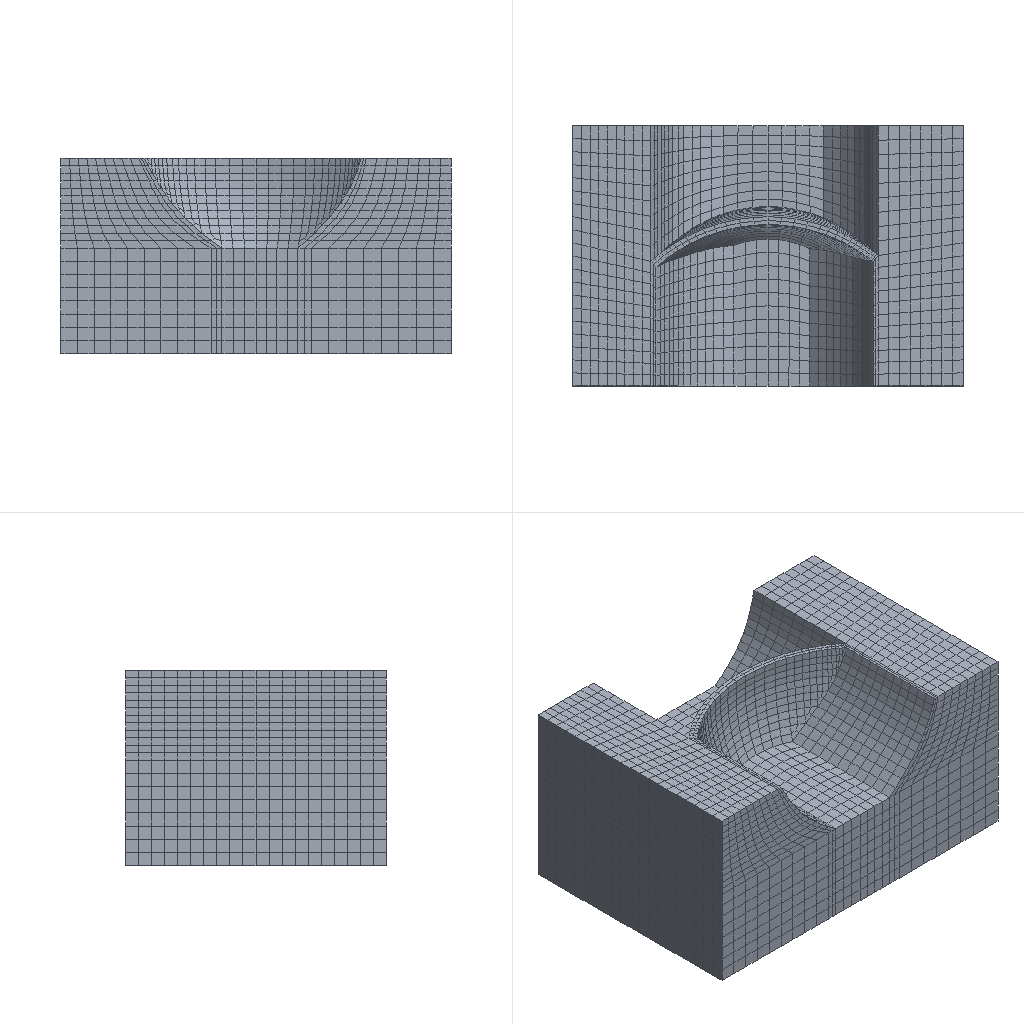Simulation study | abaqus
Set-up summary:
category,name,step,type,value,unit,region
solver,abaqus
solver,version,,,Abaqus/Standard 2020
units,not stated in the deck,,not stated
analysis,deck,,static,static
load_step,Step-1,Step-1,static
load_step,requested,,,1
mesh,nodes,,,11349
mesh,elements,,,9392
element_type,C3D8R,,solid,9392
load,load commands in deck,,count,275
bc,support commands in deck,,count,1
material,MAT-BAJI,,in results
material,MAT-BATI,,in results
check,setup vs results,,match,"per instance, exact: element labels, types and connectivity; labels of the nodes the elements use; coordinates of those nodes at SINGLE_PRECISION in 1 of 1 instance(s)"
Abaqus input file, long lists of numbers shortened:
*Heading
** Job name: Job-1 Model name: model-mesh
** Generated by: Abaqus/CAE 2020
*Preprint, echo=NO, model=NO, history=NO, contact=NO
**
** PARTS
**
*Part, name=Part-10
*Node
      1,  -79.508,  -35.548,         57.5
      2,  -80.694,  -34.215,          69.
** (11347 more lines like these left out)
*Element, type=C3D8R
1, 1819,  221, 1818, 6648,  219,    1,  220, 1817
2, 1818,  223, 1820, 6648,  220,    2,  222, 1817
** (9390 more lines like these left out)
*Nset, nset=bati
     1,     2,     3,     4,     5,     6,     7,     8,     9,    10,    11,    12,    13,    14,    15,    16
    17,    18,    19,    20,    21,    22,    23,    24,    25,    26,    27,    28,    29,    30,    31,    32
** (49 more lines like these left out)
*Elset, elset=bati
    1,    2,    3,    4,    5,    6,    7,    8,    9,   10,   11,   12,   13,   14,   15,   16
   17,   18,   19,   20,   21,   22,   23,   24,   25,   26,   27,   28,   29,   30,   31,   32
** (28 more lines like these left out)
*Nset, nset=baji
     1,     3,     5,     6,    15,    16,    26,    27,    38,    39,    52,    53,    68,    69,    70,    71
    72,    74,    75,    77,    98,    99,   108,   109,   117,   118,   121,   124,   127,   128,   129,   130
** (663 more lines like these left out)
*Elset, elset=baji, generate
  469,  9380,     1
** Section: Sec-bati
*Solid Section, elset=bati, material=Mat-bati
,
** Section: Sec-baji
*Solid Section, elset=baji, material=Mat-baji
,
*End Part
**
*Part, name=crack
*End Part
**
**
** ASSEMBLY
**
*Assembly, name=Assembly
**
*Instance, name=Part-10-1, part=Part-10
*End Instance
**
*Instance, name=crack-1, part=crack
23.198,       4.068, 38.045
23.198,       4.068, 38.045, 23.198, 5.068, 38.045, 80.
*End Instance
**
*Nset, nset=Set-9, instance=Part-10-1
    4,    5,    6,    7,   10,   11,   14,   15,   17,   20,   21,   23,   24,   26,   29,   30
   33,   34,   37,   38,   40,   42,   45,   46,   48,   50,   52,   55,   56,   59,   60,   63
** (15 more lines like these left out)
*Elset, elset=Set-9, instance=Part-10-1
    4,    5,    6,    7,    9,   11,   13,   16,   18,   20,   22,   23,   24,   25,   29,   31
   33,   35,   37,   39,   41,   43,   45,   47,   49,   51,   53,   54,   55,   59,   61,   63
** (13 more lines like these left out)
*Nset, nset=Set-10, instance=Part-10-1
    1,    2,    3,    4,    6,    8,    9,   10,   12,   13,   14,   16,   18,   19,   22,   25
   27,   28,   29,   31,   32,   33,   35,   36,   39,   41,   43,   44,   47,   49,   51,   53
** (19 more lines like these left out)
*Elset, elset=Set-10, instance=Part-10-1
    1,    2,    3,    4,    6,    8,    9,   10,   12,   13,   14,   15,   17,   19,   20,   21
   22,   26,   27,   28,   30,   32,   34,   36,   38,   40,   42,   44,   46,   48,   50,   52
** (15 more lines like these left out)
*Nset, nset=Set-11, instance=Part-10-1
     1,     2,     3,     4,     5,     6,     7,     8,     9,    10,    11,    12,    13,    14,    15,    16
    17,    18,    19,    20,    21,    22,    23,    24,    25,    26,    27,    28,    29,    30,    31,    32
** (49 more lines like these left out)
*Elset, elset=Set-11, instance=Part-10-1
    1,    2,    3,    4,    5,    6,    7,    8,    9,   10,   11,   12,   13,   14,   15,   16
   17,   18,   19,   20,   21,   22,   23,   24,   25,   26,   27,   28,   29,   30,   31,   32
** (34 more lines like these left out)
*Nset, nset=Set-14, instance=Part-10-1
  131,  132,  133,  134,  136,  137,  138,  139,  140,  142,  143,  145,  146,  150,  152,  154
  157,  158,  576,  577,  578,  579,  580,  581,  582,  583,  584,  585,  586,  587,  588,  589
** (35 more lines like these left out)
*Elset, elset=Set-14, instance=Part-10-1
  700,  701,  702,  703,  704,  705,  706,  707,  708,  709,  710,  711,  712,  713,  714,  715
  716,  717,  718,  719,  720,  721,  722,  723,  724,  725,  726,  727,  728,  729,  730,  731
** (32 more lines like these left out)
*Nset, nset=Set-15, instance=Part-10-1
    4,    5,    6,    7,   10,   11,   14,   15,   17,   20,   21,   23,   24,   26,   29,   30
   33,   34,   37,   38,   40,   42,   45,   46,   48,   50,   52,   55,   56,   59,   60,   63
** (15 more lines like these left out)
*Elset, elset=Set-15, instance=Part-10-1
    4,    5,    6,    7,    9,   11,   13,   16,   18,   20,   22,   23,   24,   25,   29,   31
   33,   35,   37,   39,   41,   43,   45,   47,   49,   51,   53,   54,   55,   59,   61,   63
** (14 more lines like these left out)
*Nset, nset=_PickedSet157, internal, instance=Part-10-1, generate
     1,  11349,      1
*Elset, elset=_PickedSet157, internal, instance=Part-10-1, generate
    1,  9392,     1
*Elset, elset=_Surf-5_S3, internal, instance=Part-10-1
   4,   6,  94, 191, 192, 195, 196, 199, 200, 214, 255, 256, 259, 260, 263, 264
 267, 268, 373, 374, 377, 378, 393, 431, 432, 467
*Elset, elset=_Surf-5_S4, internal, instance=Part-10-1
   5,  16,  18,  20,  22,  95,  96, 215, 224, 226, 228, 230, 232, 234, 236, 238
 240, 242, 244, 246, 248, 250, 252, 254, 358, 360, 362, 364, 382, 384, 386, 388
** (1 more lines like these left out)
*Elset, elset=_Surf-5_S6, internal, instance=Part-10-1
    7,    9,   11,   13,   29,   31,   33,   35,   37,   39,   41,   43,   45,   47,   49,   51
   59,   61,   63,   65,   67,   69,   71,   73,   75,   77,   79,   81,   83,   85,   87,   89
** (7 more lines like these left out)
*Elset, elset=_Surf-5_S2, internal, instance=Part-10-1
  23,  24,  25,  53,  54,  55, 137, 138, 139, 216, 217, 218, 219, 351, 352, 353
 457, 458, 459
*Elset, elset=_Surf-5_S1, internal, instance=Part-10-1, generate
 343,  350,    1
*Elset, elset=_Surf-5_S5, internal, instance=Part-10-1
 443, 444, 447, 448
*Surface, type=ELEMENT, name=Surf-5
_Surf-5_S3, S3
_Surf-5_S4, S4
_Surf-5_S6, S6
_Surf-5_S2, S2
_Surf-5_S1, S1
_Surf-5_S5, S5
*Enrichment, name=Crack-1, type=PROPAGATION CRACK, elset=_PickedSet157
*End Assembly
*Amplitude, name=Amp-1
             0.,              0.,             10.,              1.
**
** MATERIALS
**
*Material, name=Mat-baji
*Density
2770.,
*Elastic
 2.55e+10, 0.32
*Expansion
 1e-05,
*Fluid Leakoff
 1e-14, 1e-14
*Gap Flow
 0.001,
*Permeability, specific=9800.
 5.26e-09, 0.01
*Material, name=Mat-bati
*Damage Initiation, criterion=MAXPS, position=CRACKTIP
 2.5e+06,
*Damage Evolution, type=DISPLACEMENT
1.,
*Damage Stabilization
1e-05
*Density
2400.,
*Elastic
 2.55e+10, 0.2
*Expansion
 1e-05,
*Fluid Leakoff
 1e-14, 1e-14
*Gap Flow
 0.001,
*Permeability, specific=9800.
 5.26e-09, 0.01
**
** INTERACTION PROPERTIES
**
*Surface Interaction, name=IntProp-1
1.,
*Initial Conditions, type=ENRICHMENT
Part-10-1.281, 1,Crack-1, 5.75, 9.091
Part-10-1.281, 2,Crack-1, 5.75, 6.537
Part-10-1.281, 3,Crack-1, 1e-06, -4.361
Part-10-1.281, 4,Crack-1, 1e-06, 0.4588
Part-10-1.281, 5,Crack-1, -5.75, -1.695
Part-10-1.281, 6,Crack-1, -5.75, -3.416
Part-10-1.281, 7,Crack-1, 1e-06, 0.
Part-10-1.281, 8,Crack-1, 1e-06, 0.3126
Part-10-1.277, 1,Crack-1, -5.75, -1.695
Part-10-1.277, 2,Crack-1, -5.75, -3.416
Part-10-1.277, 3,Crack-1, 1e-06, 0.
Part-10-1.277, 4,Crack-1, 1e-06, 0.3126
Part-10-1.277, 5,Crack-1, -10.983, -12.704
Part-10-1.277, 6,Crack-1, -11.835, -13.569
Part-10-1.277, 7,Crack-1, -10.798, -13.53
Part-10-1.277, 8,Crack-1, -10.039, -12.759
**
** BOUNDARY CONDITIONS
**
** Name: BC-1 Type: 对称/反对称/完全固定
*Boundary
Set-14, ENCASTRE
**
** PREDEFINED FIELDS
**
** Name: Predefined Field-3   Type: Temperature
*Initial Conditions, type=TEMPERATURE
Set-11, 20.
** Name: Predefined Field-4   Type: Void ratio
*Initial Conditions, TYPE=RATIO
Part-10-1.bati, 0.7
** Name: Predefined Field-5   Type: Void ratio
*Initial Conditions, TYPE=RATIO
Part-10-1.baji, 0.4
**
** INTERACTIONS
**
** Interaction: Int-1
*Contact
*Contact Inclusions, ALL EXTERIOR
*Contact Property Assignment
 ,  , IntProp-1
** ----------------------------------------------------------------
**
** STEP: Step-1
**
*Step, name=Step-1, nlgeom=YES, inc=1000
*Static, stabilize=0.0002, allsdtol=0.05, continue=NO
0.01, 1., 1e-05, 1.
**
** LOADS
**
** Name: Load-2   Type: Pressure
*Dsload
Surf-5, HP, 676200., 69., 0.
** Name: Load-4   Type: Gravity
*Dload
, GRAV, 9.8, 0., 0., -1.
**
** PREDEFINED FIELDS
**
** Name: Predefined Field-1   Type: Temperature Using Field: T-shangyou
*Temperature
Part-10-1.4, 32.
Part-10-1.5, 28.667
Part-10-1.6, 32.
Part-10-1.7, 28.667
Part-10-1.10, 32.
Part-10-1.11, 28.667
Part-10-1.14, 32.
Part-10-1.15, 25.333
Part-10-1.17, 25.333
Part-10-1.20, 28.667
Part-10-1.21, 25.333
Part-10-1.23, 28.667
Part-10-1.24, 22.
Part-10-1.26, 22.
Part-10-1.29, 32.
Part-10-1.30, 28.667
Part-10-1.33, 32.
Part-10-1.34, 22.
Part-10-1.37, 25.333
Part-10-1.38, 18.667
Part-10-1.40, 18.667
Part-10-1.42, 25.333
Part-10-1.45, 28.667
Part-10-1.46, 22.
Part-10-1.48, 18.667
Part-10-1.50, 15.333
Part-10-1.52, 15.333
Part-10-1.55, 32.
Part-10-1.56, 28.667
Part-10-1.59, 32.
Part-10-1.60, 22.
Part-10-1.63, 25.333
Part-10-1.64, 18.667
Part-10-1.66, 15.333
Part-10-1.68, 12.
Part-10-1.70, 12.
Part-10-1.72, 12.
Part-10-1.73, 15.333
Part-10-1.74, 15.333
Part-10-1.79, 22.
** (232 more lines like these left out)
** Name: Predefined Field-2   Type: Temperature
*Temperature
Set-10, 1.
**
** INTERACTIONS
**
** Interaction: Int-2
*Enrichment Activation, name=Crack-1, activate=ON
**
** CONTROLS
**
*Controls, reset
*Controls, parameters=time incrementation
, , , , , , , 20, , ,
**
** OUTPUT REQUESTS
**
*Restart, write, frequency=0
**
** FIELD OUTPUT: F-Output-1
**
*Output, field
*Node Output
CF, NT, PHILSM, PSILSM, RF, U, V
*Element Output, directions=YES
E, HP, LE, MISES, PE, PEEQ, PEMAG, RD, S, SDEG, TEMP
*Contact Output
CDISP, CSTRESS, PPRESS
**
** HISTORY OUTPUT: H-Output-1
**
*Output, history, variable=PRESELECT
*End Step
Results summary:
result,step,,completed,increments=11 time=1.0/1.0
result,analysis,,,static
result,last_loadstep,,,1
result,primary field,,,U
result,reaction total,,FX,31116310.5,model units
result,reaction total,,FY,2901110474.125,model units
result,reaction total,,FZ,198232237408.0,model units